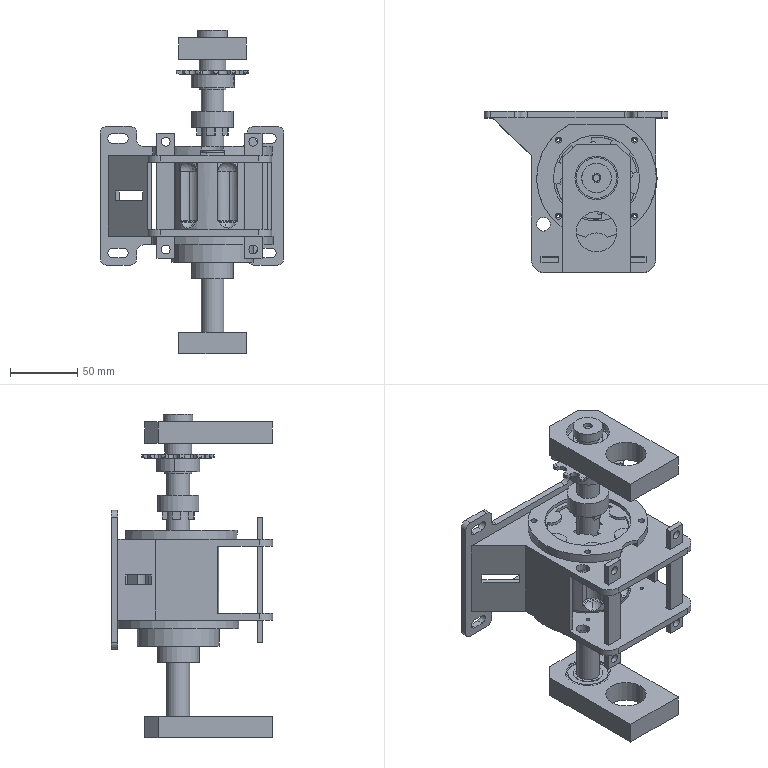Part | NX | features EXTRUDE 21, DATUM_CSYS 11, SKETCH 11, LINKED_FACE 6, BREP 5, UNITE 5, EXTRACT_DATUM_PLANE 4, EXTRACT_BODY 3, CHAMFER 2, INTERSECT 2, LINKED_BODY 1, Pattern Geometry 1, REPLACE_FACE 1 | 17 solids | 598 faces | box 136.5 x 120 x 240 mm | volume 520040 mm3 | plane 287 | cylinder 237 | cone 26 | torus 24 | sphere 18 | spline 6 | commonest cylinder face diameters 20 x32 7.77 x17 2.5 x16 16 x16 30 x14 17 x13